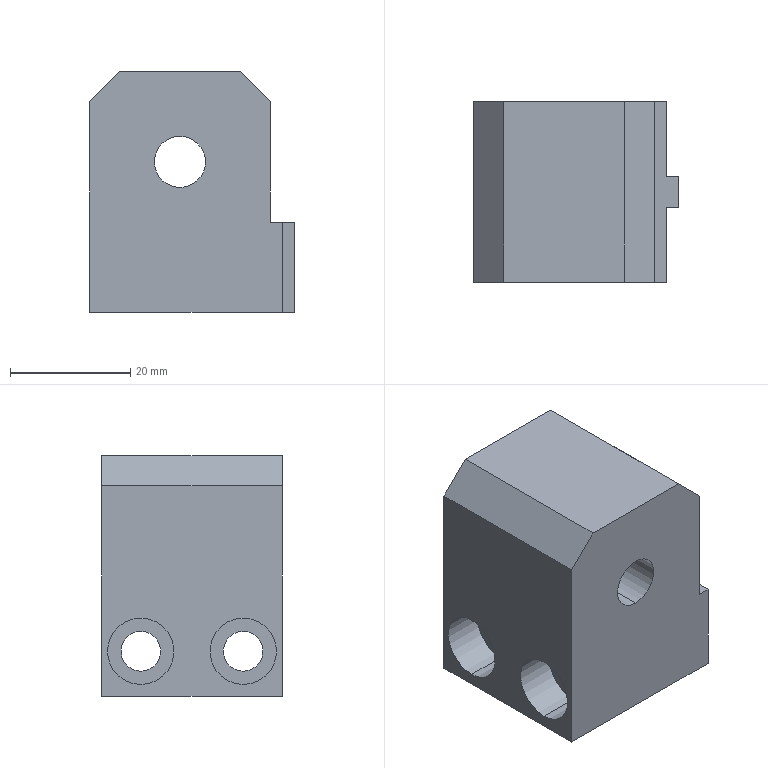Part | SolidWorks | features BaseBody 1 | 1 solid | 26 faces | box 34 x 30 x 40 mm | volume 31581 mm3 | plane 16 | cylinder 10 | commonest cylinder face diameters 6.6 x4 11 x4 8.5 x2
STEP:
#1=CARTESIAN_POINT('',(-34.,30.,35.));
#2=VERTEX_POINT('',#1);
#3=CARTESIAN_POINT('',(-29.,30.,40.));
#4=VERTEX_POINT('',#3);
#5=CARTESIAN_POINT('',(-29.,30.,40.));
#6=DIRECTION('',(0.7071,0.,0.7071));
#7=VECTOR('',#6,1000.);
#8=LINE('',#5,#7);
#9=EDGE_CURVE('',#2,#4,#8,.T.);
#10=ORIENTED_EDGE('',*,*,#9,.F.);
#11=CARTESIAN_POINT('',(-34.,0.,35.));
#12=VERTEX_POINT('',#11);
#13=CARTESIAN_POINT('',(-34.,30.,35.));
#14=DIRECTION('',(0.,1.,0.));
#15=VECTOR('',#14,1000.);
#16=LINE('',#13,#15);
#17=EDGE_CURVE('',#12,#2,#16,.T.);
#18=ORIENTED_EDGE('',*,*,#17,.F.);
#19=CARTESIAN_POINT('',(-29.,0.,40.));
#20=VERTEX_POINT('',#19);
#21=CARTESIAN_POINT('',(-34.5,0.,34.5));
#22=DIRECTION('',(-0.7071,0.,-0.7071));
#23=VECTOR('',#22,1000.);
#24=LINE('',#21,#23);
#25=EDGE_CURVE('',#20,#12,#24,.T.);
#26=ORIENTED_EDGE('',*,*,#25,.F.);
#27=CARTESIAN_POINT('',(-29.,30.,40.));
#28=DIRECTION('',(0.,-1.,0.));
#29=VECTOR('',#28,1000.);
#30=LINE('',#27,#29);
#31=EDGE_CURVE('',#4,#20,#30,.T.);
#32=ORIENTED_EDGE('',*,*,#31,.F.);
#33=EDGE_LOOP('',(#10,#18,#26,#32));
#34=FACE_OUTER_BOUND('',#33,.T.);
#35=CARTESIAN_POINT('',(-29.,30.,40.));
#36=DIRECTION('',(0.7071,0.,-0.7071));
#37=DIRECTION('',(0.,-1.,0.));
#38=AXIS2_PLACEMENT_3D('',#35,#36,#37);
#39=PLANE('',#38);
#40=ADVANCED_FACE('',(#34),#39,.F.);
#41=CARTESIAN_POINT('',(-9.,30.,40.));
#42=VERTEX_POINT('',#41);
#43=CARTESIAN_POINT('',(-4.,30.,35.));
#44=VERTEX_POINT('',#43);
#45=CARTESIAN_POINT('',(-4.,30.,35.));
#46=DIRECTION('',(0.7071,0.,-0.7071));
#47=VECTOR('',#46,1000.);
#48=LINE('',#45,#47);
#49=EDGE_CURVE('',#42,#44,#48,.T.);
#50=ORIENTED_EDGE('',*,*,#49,.F.);
#51=CARTESIAN_POINT('',(-9.,0.,40.));
#52=VERTEX_POINT('',#51);
#53=CARTESIAN_POINT('',(-9.,30.,40.));
#54=DIRECTION('',(0.,1.,0.));
#55=VECTOR('',#54,1000.);
#56=LINE('',#53,#55);
#57=EDGE_CURVE('',#52,#42,#56,.T.);
#58=ORIENTED_EDGE('',*,*,#57,.F.);
#59=CARTESIAN_POINT('',(-4.,0.,35.));
#60=VERTEX_POINT('',#59);
#61=CARTESIAN_POINT('',(15.5,0.,15.5));
#62=DIRECTION('',(-0.7071,0.,0.7071));
#63=VECTOR('',#62,1000.);
#64=LINE('',#61,#63);
#65=EDGE_CURVE('',#60,#52,#64,.T.);
#66=ORIENTED_EDGE('',*,*,#65,.F.);
#67=CARTESIAN_POINT('',(-4.,30.,35.));
#68=DIRECTION('',(0.,-1.,0.));
#69=VECTOR('',#68,1000.);
#70=LINE('',#67,#69);
#71=EDGE_CURVE('',#44,#60,#70,.T.);
#72=ORIENTED_EDGE('',*,*,#71,.F.);
#73=EDGE_LOOP('',(#50,#58,#66,#72));
#74=FACE_OUTER_BOUND('',#73,.T.);
#75=CARTESIAN_POINT('',(-4.,30.,35.));
#76=DIRECTION('',(-0.7071,0.,-0.7071));
#77=DIRECTION('',(-0.7071,0.,0.7071));
#78=AXIS2_PLACEMENT_3D('',#75,#76,#77);
#79=PLANE('',#78);
#80=ADVANCED_FACE('',(#74),#79,.F.);
#81=CARTESIAN_POINT('',(-27.2,23.5,2.));
#82=VERTEX_POINT('',#81);
#83=CARTESIAN_POINT('',(-34.,23.5,2.));
#84=VERTEX_POINT('',#83);
#85=CARTESIAN_POINT('',(-34.,23.5,2.));
#86=DIRECTION('',(-1.,0.,0.));
#87=VECTOR('',#86,1000.);
#88=LINE('',#85,#87);
#89=EDGE_CURVE('',#82,#84,#88,.T.);
#90=ORIENTED_EDGE('',*,*,#89,.F.);
#91=CARTESIAN_POINT('',(-27.2,23.5,13.));
#92=VERTEX_POINT('',#91);
#93=CARTESIAN_POINT('',(-27.2,23.5,7.5));
#94=DIRECTION('',(-1.,0.,0.));
#95=DIRECTION('',(0.,0.,1.));
#96=AXIS2_PLACEMENT_3D('',#93,#94,#95);
#97=CIRCLE('',#96,5.5);
#98=EDGE_CURVE('',#92,#82,#97,.T.);
#99=ORIENTED_EDGE('',*,*,#98,.F.);
#100=CARTESIAN_POINT('',(-34.,23.5,13.));
#101=VERTEX_POINT('',#100);
#102=CARTESIAN_POINT('',(-34.,23.5,13.));
#103=DIRECTION('',(-1.,0.,0.));
#104=VECTOR('',#103,1000.);
#105=LINE('',#102,#104);
#106=EDGE_CURVE('',#92,#101,#105,.T.);
#107=ORIENTED_EDGE('',*,*,#106,.T.);
#108=CARTESIAN_POINT('',(-34.,23.5,7.5));
#109=DIRECTION('',(-1.,0.,0.));
#110=DIRECTION('',(0.,0.,1.));
#111=AXIS2_PLACEMENT_3D('',#108,#109,#110);
#112=CIRCLE('',#111,5.5);
#113=EDGE_CURVE('',#101,#84,#112,.T.);
#114=ORIENTED_EDGE('',*,*,#113,.T.);
#115=EDGE_LOOP('',(#90,#99,#107,#114));
#116=FACE_OUTER_BOUND('',#115,.T.);
#117=CARTESIAN_POINT('',(-34.,23.5,7.5));
#118=DIRECTION('',(-1.,0.,0.));
#119=DIRECTION('',(0.,0.,1.));
#120=AXIS2_PLACEMENT_3D('',#117,#118,#119);
#121=CYLINDRICAL_SURFACE('',#120,5.5);
#122=ADVANCED_FACE('',(#116),#121,.F.);
#123=CARTESIAN_POINT('',(-27.2,23.5,10.8));
#124=VERTEX_POINT('',#123);
#125=CARTESIAN_POINT('',(-27.2,23.5,4.2));
#126=VERTEX_POINT('',#125);
#127=CARTESIAN_POINT('',(-27.2,23.5,7.5));
#128=DIRECTION('',(-1.,0.,0.));
#129=DIRECTION('',(0.,0.,1.));
#130=AXIS2_PLACEMENT_3D('',#127,#128,#129);
#131=CIRCLE('',#130,3.3);
#132=EDGE_CURVE('',#124,#126,#131,.T.);
#133=ORIENTED_EDGE('',*,*,#132,.F.);
#134=CARTESIAN_POINT('',(-27.2,23.5,7.5));
#135=DIRECTION('',(-1.,0.,0.));
#136=DIRECTION('',(0.,0.,1.));
#137=AXIS2_PLACEMENT_3D('',#134,#135,#136);
#138=CIRCLE('',#137,3.3);
#139=EDGE_CURVE('',#126,#124,#138,.T.);
#140=ORIENTED_EDGE('',*,*,#139,.F.);
#141=EDGE_LOOP('',(#133,#140));
#142=FACE_BOUND('',#141,.T.);
#143=ORIENTED_EDGE('',*,*,#98,.T.);
#144=CARTESIAN_POINT('',(-27.2,23.5,7.5));
#145=DIRECTION('',(-1.,0.,0.));
#146=DIRECTION('',(0.,0.,1.));
#147=AXIS2_PLACEMENT_3D('',#144,#145,#146);
#148=CIRCLE('',#147,5.5);
#149=EDGE_CURVE('',#82,#92,#148,.T.);
#150=ORIENTED_EDGE('',*,*,#149,.T.);
#151=EDGE_LOOP('',(#143,#150));
#152=FACE_OUTER_BOUND('',#151,.T.);
#153=CARTESIAN_POINT('',(-27.2,26.8,7.5));
#154=DIRECTION('',(1.,0.,0.));
#155=DIRECTION('',(0.,0.,-1.));
#156=AXIS2_PLACEMENT_3D('',#153,#154,#155);
#157=PLANE('',#156);
#158=ADVANCED_FACE('',(#142,#152),#157,.F.);
#159=CARTESIAN_POINT('',(-2.,23.5,4.2));
#160=VERTEX_POINT('',#159);
#161=CARTESIAN_POINT('',(-34.,23.5,4.2));
#162=DIRECTION('',(-1.,0.,0.));
#163=VECTOR('',#162,1000.);
#164=LINE('',#161,#163);
#165=EDGE_CURVE('',#160,#126,#164,.T.);
#166=ORIENTED_EDGE('',*,*,#165,.F.);
#167=CARTESIAN_POINT('',(-2.,23.5,10.8));
#168=VERTEX_POINT('',#167);
#169=CARTESIAN_POINT('',(-2.,23.5,7.5));
#170=DIRECTION('',(1.,0.,0.));
#171=DIRECTION('',(0.,0.,-1.));
#172=AXIS2_PLACEMENT_3D('',#169,#170,#171);
#173=CIRCLE('',#172,3.3);
#174=EDGE_CURVE('',#160,#168,#173,.T.);
#175=ORIENTED_EDGE('',*,*,#174,.T.);
#176=CARTESIAN_POINT('',(-34.,23.5,10.8));
#177=DIRECTION('',(-1.,0.,0.));
#178=VECTOR('',#177,1000.);
#179=LINE('',#176,#178);
#180=EDGE_CURVE('',#168,#124,#179,.T.);
#181=ORIENTED_EDGE('',*,*,#180,.T.);
#182=ORIENTED_EDGE('',*,*,#132,.T.);
#183=EDGE_LOOP('',(#166,#175,#181,#182));
#184=FACE_OUTER_BOUND('',#183,.T.);
#185=CARTESIAN_POINT('',(-34.,23.5,7.5));
#186=DIRECTION('',(-1.,0.,0.));
#187=DIRECTION('',(0.,0.,1.));
#188=AXIS2_PLACEMENT_3D('',#185,#186,#187);
#189=CYLINDRICAL_SURFACE('',#188,3.3);
#190=ADVANCED_FACE('',(#184),#189,.F.);
#191=CARTESIAN_POINT('',(-27.2,6.5,2.));
#192=VERTEX_POINT('',#191);
#193=CARTESIAN_POINT('',(-34.,6.5,2.));
#194=VERTEX_POINT('',#193);
#195=CARTESIAN_POINT('',(-34.,6.5,2.));
#196=DIRECTION('',(-1.,0.,0.));
#197=VECTOR('',#196,1000.);
#198=LINE('',#195,#197);
#199=EDGE_CURVE('',#192,#194,#198,.T.);
#200=ORIENTED_EDGE('',*,*,#199,.F.);
#201=CARTESIAN_POINT('',(-27.2,6.5,13.));
#202=VERTEX_POINT('',#201);
#203=CARTESIAN_POINT('',(-27.2,6.5,7.5));
#204=DIRECTION('',(-1.,0.,0.));
#205=DIRECTION('',(0.,0.,1.));
#206=AXIS2_PLACEMENT_3D('',#203,#204,#205);
#207=CIRCLE('',#206,5.5);
#208=EDGE_CURVE('',#202,#192,#207,.T.);
#209=ORIENTED_EDGE('',*,*,#208,.F.);
#210=CARTESIAN_POINT('',(-34.,6.5,13.));
#211=VERTEX_POINT('',#210);
#212=CARTESIAN_POINT('',(-34.,6.5,13.));
#213=DIRECTION('',(-1.,0.,0.));
#214=VECTOR('',#213,1000.);
#215=LINE('',#212,#214);
#216=EDGE_CURVE('',#202,#211,#215,.T.);
#217=ORIENTED_EDGE('',*,*,#216,.T.);
#218=CARTESIAN_POINT('',(-34.,6.5,7.5));
#219=DIRECTION('',(-1.,0.,0.));
#220=DIRECTION('',(0.,0.,1.));
#221=AXIS2_PLACEMENT_3D('',#218,#219,#220);
#222=CIRCLE('',#221,5.5);
#223=EDGE_CURVE('',#211,#194,#222,.T.);
#224=ORIENTED_EDGE('',*,*,#223,.T.);
#225=EDGE_LOOP('',(#200,#209,#217,#224));
#226=FACE_OUTER_BOUND('',#225,.T.);
#227=CARTESIAN_POINT('',(-34.,6.5,7.5));
#228=DIRECTION('',(-1.,0.,0.));
#229=DIRECTION('',(0.,0.,1.));
#230=AXIS2_PLACEMENT_3D('',#227,#228,#229);
#231=CYLINDRICAL_SURFACE('',#230,5.5);
#232=ADVANCED_FACE('',(#226),#231,.F.);
#233=CARTESIAN_POINT('',(-27.2,6.5,10.8));
#234=VERTEX_POINT('',#233);
#235=CARTESIAN_POINT('',(-27.2,6.5,4.2));
#236=VERTEX_POINT('',#235);
#237=CARTESIAN_POINT('',(-27.2,6.5,7.5));
#238=DIRECTION('',(-1.,0.,0.));
#239=DIRECTION('',(0.,0.,1.));
#240=AXIS2_PLACEMENT_3D('',#237,#238,#239);
#241=CIRCLE('',#240,3.3);
#242=EDGE_CURVE('',#234,#236,#241,.T.);
#243=ORIENTED_EDGE('',*,*,#242,.F.);
#244=CARTESIAN_POINT('',(-27.2,6.5,7.5));
#245=DIRECTION('',(-1.,0.,0.));
#246=DIRECTION('',(0.,0.,1.));
#247=AXIS2_PLACEMENT_3D('',#244,#245,#246);
#248=CIRCLE('',#247,3.3);
#249=EDGE_CURVE('',#236,#234,#248,.T.);
#250=ORIENTED_EDGE('',*,*,#249,.F.);
#251=EDGE_LOOP('',(#243,#250));
#252=FACE_BOUND('',#251,.T.);
#253=ORIENTED_EDGE('',*,*,#208,.T.);
#254=CARTESIAN_POINT('',(-27.2,6.5,7.5));
#255=DIRECTION('',(-1.,0.,0.));
#256=DIRECTION('',(0.,0.,1.));
#257=AXIS2_PLACEMENT_3D('',#254,#255,#256);
#258=CIRCLE('',#257,5.5);
#259=EDGE_CURVE('',#192,#202,#258,.T.);
#260=ORIENTED_EDGE('',*,*,#259,.T.);
#261=EDGE_LOOP('',(#253,#260));
#262=FACE_OUTER_BOUND('',#261,.T.);
#263=CARTESIAN_POINT('',(-27.2,9.8,7.5));
#264=DIRECTION('',(1.,0.,0.));
#265=DIRECTION('',(0.,0.,-1.));
#266=AXIS2_PLACEMENT_3D('',#263,#264,#265);
#267=PLANE('',#266);
#268=ADVANCED_FACE('',(#252,#262),#267,.F.);
#269=CARTESIAN_POINT('',(-2.,6.5,4.2));
#270=VERTEX_POINT('',#269);
#271=CARTESIAN_POINT('',(-34.,6.5,4.2));
#272=DIRECTION('',(-1.,0.,0.));
#273=VECTOR('',#272,1000.);
#274=LINE('',#271,#273);
#275=EDGE_CURVE('',#270,#236,#274,.T.);
#276=ORIENTED_EDGE('',*,*,#275,.F.);
#277=CARTESIAN_POINT('',(-2.,6.5,10.8));
#278=VERTEX_POINT('',#277);
#279=CARTESIAN_POINT('',(-2.,6.5,7.5));
#280=DIRECTION('',(1.,0.,0.));
#281=DIRECTION('',(0.,0.,-1.));
#282=AXIS2_PLACEMENT_3D('',#279,#280,#281);
#283=CIRCLE('',#282,3.3);
#284=EDGE_CURVE('',#270,#278,#283,.T.);
#285=ORIENTED_EDGE('',*,*,#284,.T.);
#286=CARTESIAN_POINT('',(-34.,6.5,10.8));
#287=DIRECTION('',(-1.,0.,0.));
#288=VECTOR('',#287,1000.);
#289=LINE('',#286,#288);
#290=EDGE_CURVE('',#278,#234,#289,.T.);
#291=ORIENTED_EDGE('',*,*,#290,.T.);
#292=ORIENTED_EDGE('',*,*,#242,.T.);
#293=EDGE_LOOP('',(#276,#285,#291,#292));
#294=FACE_OUTER_BOUND('',#293,.T.);
#295=CARTESIAN_POINT('',(-34.,6.5,7.5));
#296=DIRECTION('',(-1.,0.,0.));
#297=DIRECTION('',(0.,0.,1.));
#298=AXIS2_PLACEMENT_3D('',#295,#296,#297);
#299=CYLINDRICAL_SURFACE('',#298,3.3);
#300=ADVANCED_FACE('',(#294),#299,.F.);
#301=CARTESIAN_POINT('',(-2.,23.5,7.5));
#302=DIRECTION('',(1.,0.,0.));
#303=DIRECTION('',(0.,0.,-1.));
#304=AXIS2_PLACEMENT_3D('',#301,#302,#303);
#305=CIRCLE('',#304,3.3);
#306=EDGE_CURVE('',#168,#160,#305,.T.);
#307=ORIENTED_EDGE('',*,*,#306,.F.);
#308=ORIENTED_EDGE('',*,*,#174,.F.);
#309=EDGE_LOOP('',(#307,#308));
#310=FACE_BOUND('',#309,.T.);
#311=CARTESIAN_POINT('',(-2.,30.,15.));
#312=VERTEX_POINT('',#311);
#313=CARTESIAN_POINT('',(-2.,17.5,15.));
#314=VERTEX_POINT('',#313);
#315=CARTESIAN_POINT('',(-2.,30.,15.));
#316=DIRECTION('',(0.,-1.,0.));
#317=VECTOR('',#316,1000.);
#318=LINE('',#315,#317);
#319=EDGE_CURVE('',#312,#314,#318,.T.);
#320=ORIENTED_EDGE('',*,*,#319,.T.);
#321=CARTESIAN_POINT('',(-2.,17.5,0.));
#322=VERTEX_POINT('',#321);
#323=CARTESIAN_POINT('',(-2.,17.5,15.));
#324=DIRECTION('',(0.,0.,-1.));
#325=VECTOR('',#324,1000.);
#326=LINE('',#323,#325);
#327=EDGE_CURVE('',#314,#322,#326,.T.);
#328=ORIENTED_EDGE('',*,*,#327,.T.);
#329=CARTESIAN_POINT('',(-2.,30.,0.));
#330=VERTEX_POINT('',#329);
#331=CARTESIAN_POINT('',(-2.,30.,0.));
#332=DIRECTION('',(0.,1.,0.));
#333=VECTOR('',#332,1000.);
#334=LINE('',#331,#333);
#335=EDGE_CURVE('',#322,#330,#334,.T.);
#336=ORIENTED_EDGE('',*,*,#335,.T.);
#337=CARTESIAN_POINT('',(-2.,30.,15.));
#338=DIRECTION('',(0.,0.,1.));
#339=VECTOR('',#338,1000.);
#340=LINE('',#337,#339);
#341=EDGE_CURVE('',#330,#312,#340,.T.);
#342=ORIENTED_EDGE('',*,*,#341,.T.);
#343=EDGE_LOOP('',(#320,#328,#336,#342));
#344=FACE_OUTER_BOUND('',#343,.T.);
#345=CARTESIAN_POINT('',(-2.,0.,0.));
#346=DIRECTION('',(1.,0.,0.));
#347=DIRECTION('',(0.,0.,-1.));
#348=AXIS2_PLACEMENT_3D('',#345,#346,#347);
#349=PLANE('',#348);
#350=ADVANCED_FACE('',(#310,#344),#349,.T.);
#351=CARTESIAN_POINT('',(0.,17.5,15.));
#352=VERTEX_POINT('',#351);
#353=CARTESIAN_POINT('',(0.,17.5,0.));
#354=VERTEX_POINT('',#353);
#355=CARTESIAN_POINT('',(0.,17.5,15.));
#356=DIRECTION('',(0.,0.,-1.));
#357=VECTOR('',#356,1000.);
#358=LINE('',#355,#357);
#359=EDGE_CURVE('',#352,#354,#358,.T.);
#360=ORIENTED_EDGE('',*,*,#359,.T.);
#361=CARTESIAN_POINT('',(-2.,17.5,0.));
#362=DIRECTION('',(1.,0.,0.));
#363=VECTOR('',#362,1000.);
#364=LINE('',#361,#363);
#365=EDGE_CURVE('',#322,#354,#364,.T.);
#366=ORIENTED_EDGE('',*,*,#365,.F.);
#367=ORIENTED_EDGE('',*,*,#327,.F.);
#368=CARTESIAN_POINT('',(-2.,17.5,15.));
#369=DIRECTION('',(1.,0.,0.));
#370=VECTOR('',#369,1000.);
#371=LINE('',#368,#370);
#372=EDGE_CURVE('',#314,#352,#371,.T.);
#373=ORIENTED_EDGE('',*,*,#372,.T.);
#374=EDGE_LOOP('',(#360,#366,#367,#373));
#375=FACE_OUTER_BOUND('',#374,.T.);
#376=CARTESIAN_POINT('',(-2.,17.5,15.));
#377=DIRECTION('',(0.,-1.,0.));
#378=DIRECTION('',(0.,0.,-1.));
#379=AXIS2_PLACEMENT_3D('',#376,#377,#378);
#380=PLANE('',#379);
#381=ADVANCED_FACE('',(#375),#380,.F.);
#382=CARTESIAN_POINT('',(-2.,6.5,7.5));
#383=DIRECTION('',(1.,0.,0.));
#384=DIRECTION('',(0.,0.,-1.));
#385=AXIS2_PLACEMENT_3D('',#382,#383,#384);
#386=CIRCLE('',#385,3.3);
#387=EDGE_CURVE('',#278,#270,#386,.T.);
#388=ORIENTED_EDGE('',*,*,#387,.F.);
#389=ORIENTED_EDGE('',*,*,#284,.F.);
#390=EDGE_LOOP('',(#388,#389));
#391=FACE_BOUND('',#390,.T.);
#392=CARTESIAN_POINT('',(-2.,0.,15.));
#393=VERTEX_POINT('',#392);
#394=CARTESIAN_POINT('',(-2.,0.,0.));
#395=VERTEX_POINT('',#394);
#396=CARTESIAN_POINT('',(-2.,0.,15.));
#397=DIRECTION('',(0.,0.,-1.));
#398=VECTOR('',#397,1000.);
#399=LINE('',#396,#398);
#400=EDGE_CURVE('',#393,#395,#399,.T.);
#401=ORIENTED_EDGE('',*,*,#400,.T.);
#402=CARTESIAN_POINT('',(-2.,12.5,0.));
#403=VERTEX_POINT('',#402);
#404=CARTESIAN_POINT('',(-2.,0.,0.));
#405=DIRECTION('',(0.,1.,0.));
#406=VECTOR('',#405,1000.);
#407=LINE('',#404,#406);
#408=EDGE_CURVE('',#395,#403,#407,.T.);
#409=ORIENTED_EDGE('',*,*,#408,.T.);
#410=CARTESIAN_POINT('',(-2.,12.5,15.));
#411=VERTEX_POINT('',#410);
#412=CARTESIAN_POINT('',(-2.,12.5,15.));
#413=DIRECTION('',(0.,0.,1.));
#414=VECTOR('',#413,1000.);
#415=LINE('',#412,#414);
#416=EDGE_CURVE('',#403,#411,#415,.T.);
#417=ORIENTED_EDGE('',*,*,#416,.T.);
#418=CARTESIAN_POINT('',(-2.,0.,15.));
#419=DIRECTION('',(0.,-1.,0.));
#420=VECTOR('',#419,1000.);
#421=LINE('',#418,#420);
#422=EDGE_CURVE('',#411,#393,#421,.T.);
#423=ORIENTED_EDGE('',*,*,#422,.T.);
#424=EDGE_LOOP('',(#401,#409,#417,#423));
#425=FACE_OUTER_BOUND('',#424,.T.);
#426=CARTESIAN_POINT('',(-2.,0.,0.));
#427=DIRECTION('',(1.,0.,0.));
#428=DIRECTION('',(0.,0.,-1.));
#429=AXIS2_PLACEMENT_3D('',#426,#427,#428);
#430=PLANE('',#429);
#431=ADVANCED_FACE('',(#391,#425),#430,.T.);
#432=CARTESIAN_POINT('',(0.,12.5,0.));
#433=VERTEX_POINT('',#432);
#434=CARTESIAN_POINT('',(0.,12.5,15.));
#435=VERTEX_POINT('',#434);
#436=CARTESIAN_POINT('',(0.,12.5,15.));
#437=DIRECTION('',(0.,0.,1.));
#438=VECTOR('',#437,1000.);
#439=LINE('',#436,#438);
#440=EDGE_CURVE('',#433,#435,#439,.T.);
#441=ORIENTED_EDGE('',*,*,#440,.T.);
#442=CARTESIAN_POINT('',(-2.,12.5,15.));
#443=DIRECTION('',(1.,0.,0.));
#444=VECTOR('',#443,1000.);
#445=LINE('',#442,#444);
#446=EDGE_CURVE('',#411,#435,#445,.T.);
#447=ORIENTED_EDGE('',*,*,#446,.F.);
#448=ORIENTED_EDGE('',*,*,#416,.F.);
#449=CARTESIAN_POINT('',(-2.,12.5,0.));
#450=DIRECTION('',(1.,0.,0.));
#451=VECTOR('',#450,1000.);
#452=LINE('',#449,#451);
#453=EDGE_CURVE('',#403,#433,#452,.T.);
#454=ORIENTED_EDGE('',*,*,#453,.T.);
#455=EDGE_LOOP('',(#441,#447,#448,#454));
#456=FACE_OUTER_BOUND('',#455,.T.);
#457=CARTESIAN_POINT('',(-2.,12.5,15.));
#458=DIRECTION('',(0.,1.,0.));
#459=DIRECTION('',(0.,0.,-1.));
#460=AXIS2_PLACEMENT_3D('',#457,#458,#459);
#461=PLANE('',#460);
#462=ADVANCED_FACE('',(#456),#461,.F.);
#463=CARTESIAN_POINT('',(-19.,0.,20.75));
#464=VERTEX_POINT('',#463);
#465=CARTESIAN_POINT('',(-19.,30.,20.75));
#466=VERTEX_POINT('',#465);
#467=CARTESIAN_POINT('',(-19.,30.,20.75));
#468=DIRECTION('',(0.,1.,0.));
#469=VECTOR('',#468,1000.);
#470=LINE('',#467,#469);
#471=EDGE_CURVE('',#464,#466,#470,.T.);
#472=ORIENTED_EDGE('',*,*,#471,.F.);
#473=CARTESIAN_POINT('',(-19.,0.,29.25));
#474=VERTEX_POINT('',#473);
#475=CARTESIAN_POINT('',(-19.,0.,25.));
#476=DIRECTION('',(0.,1.,0.));
#477=DIRECTION('',(0.,0.,1.));
#478=AXIS2_PLACEMENT_3D('',#475,#476,#477);
#479=CIRCLE('',#478,4.25);
#480=EDGE_CURVE('',#474,#464,#479,.T.);
#481=ORIENTED_EDGE('',*,*,#480,.F.);
#482=CARTESIAN_POINT('',(-19.,30.,29.25));
#483=VERTEX_POINT('',#482);
#484=CARTESIAN_POINT('',(-19.,30.,29.25));
#485=DIRECTION('',(0.,1.,0.));
#486=VECTOR('',#485,1000.);
#487=LINE('',#484,#486);
#488=EDGE_CURVE('',#474,#483,#487,.T.);
#489=ORIENTED_EDGE('',*,*,#488,.T.);
#490=CARTESIAN_POINT('',(-19.,30.,25.));
#491=DIRECTION('',(0.,1.,0.));
#492=DIRECTION('',(0.,0.,1.));
#493=AXIS2_PLACEMENT_3D('',#490,#491,#492);
#494=CIRCLE('',#493,4.25);
#495=EDGE_CURVE('',#483,#466,#494,.T.);
#496=ORIENTED_EDGE('',*,*,#495,.T.);
#497=EDGE_LOOP('',(#472,#481,#489,#496));
#498=FACE_OUTER_BOUND('',#497,.T.);
#499=CARTESIAN_POINT('',(-19.,30.,25.));
#500=DIRECTION('',(0.,1.,0.));
#501=DIRECTION('',(0.,0.,1.));
#502=AXIS2_PLACEMENT_3D('',#499,#500,#501);
#503=CYLINDRICAL_SURFACE('',#502,4.25);
#504=ADVANCED_FACE('',(#498),#503,.F.);
#505=CARTESIAN_POINT('',(0.,30.,15.));
#506=DIRECTION('',(0.,-1.,0.));
#507=VECTOR('',#506,1000.);
#508=LINE('',#505,#507);
#509=EDGE_CURVE('',#352,#435,#508,.T.);
#510=ORIENTED_EDGE('',*,*,#509,.F.);
#511=ORIENTED_EDGE('',*,*,#372,.F.);
#512=ORIENTED_EDGE('',*,*,#319,.F.);
#513=CARTESIAN_POINT('',(-4.,30.,15.));
#514=VERTEX_POINT('',#513);
#515=CARTESIAN_POINT('',(0.,30.,15.));
#516=DIRECTION('',(1.,0.,0.));
#517=VECTOR('',#516,1000.);
#518=LINE('',#515,#517);
#519=EDGE_CURVE('',#514,#312,#518,.T.);
#520=ORIENTED_EDGE('',*,*,#519,.F.);
#521=CARTESIAN_POINT('',(-4.,0.,15.));
#522=VERTEX_POINT('',#521);
#523=CARTESIAN_POINT('',(-4.,30.,15.));
#524=DIRECTION('',(0.,-1.,0.));
#525=VECTOR('',#524,1000.);
#526=LINE('',#523,#525);
#527=EDGE_CURVE('',#514,#522,#526,.T.);
#528=ORIENTED_EDGE('',*,*,#527,.T.);
#529=CARTESIAN_POINT('',(0.,0.,15.));
#530=DIRECTION('',(1.,0.,0.));
#531=VECTOR('',#530,1000.);
#532=LINE('',#529,#531);
#533=EDGE_CURVE('',#522,#393,#532,.T.);
#534=ORIENTED_EDGE('',*,*,#533,.T.);
#535=ORIENTED_EDGE('',*,*,#422,.F.);
#536=ORIENTED_EDGE('',*,*,#446,.T.);
#537=EDGE_LOOP('',(#510,#511,#512,#520,#528,#534,#535,#536));
#538=FACE_OUTER_BOUND('',#537,.T.);
#539=CARTESIAN_POINT('',(0.,30.,15.));
#540=DIRECTION('',(0.,0.,-1.));
#541=DIRECTION('',(0.,-1.,0.));
#542=AXIS2_PLACEMENT_3D('',#539,#540,#541);
#543=PLANE('',#542);
#544=ADVANCED_FACE('',(#538),#543,.F.);
#545=CARTESIAN_POINT('',(-4.,30.,15.));
#546=DIRECTION('',(0.,0.,-1.));
#547=VECTOR('',#546,1000.);
#548=LINE('',#545,#547);
#549=EDGE_CURVE('',#44,#514,#548,.T.);
#550=ORIENTED_EDGE('',*,*,#549,.F.);
#551=ORIENTED_EDGE('',*,*,#71,.T.);
#552=CARTESIAN_POINT('',(-4.,0.,15.));
#553=DIRECTION('',(0.,0.,-1.));
#554=VECTOR('',#553,1000.);
#555=LINE('',#552,#554);
#556=EDGE_CURVE('',#60,#522,#555,.T.);
#557=ORIENTED_EDGE('',*,*,#556,.T.);
#558=ORIENTED_EDGE('',*,*,#527,.F.);
#559=EDGE_LOOP('',(#550,#551,#557,#558));
#560=FACE_OUTER_BOUND('',#559,.T.);
#561=CARTESIAN_POINT('',(-4.,30.,15.));
#562=DIRECTION('',(-1.,0.,0.));
#563=DIRECTION('',(0.,1.,0.));
#564=AXIS2_PLACEMENT_3D('',#561,#562,#563);
#565=PLANE('',#564);
#566=ADVANCED_FACE('',(#560),#565,.F.);
#567=CARTESIAN_POINT('',(-34.,0.,40.));
#568=DIRECTION('',(1.,0.,0.));
#569=VECTOR('',#568,1000.);
#570=LINE('',#567,#569);
#571=EDGE_CURVE('',#20,#52,#570,.T.);
#572=ORIENTED_EDGE('',*,*,#571,.T.);
#573=ORIENTED_EDGE('',*,*,#57,.T.);
#574=CARTESIAN_POINT('',(-34.,30.,40.));
#575=DIRECTION('',(1.,0.,0.));
#576=VECTOR('',#575,1000.);
#577=LINE('',#574,#576);
#578=EDGE_CURVE('',#4,#42,#577,.T.);
#579=ORIENTED_EDGE('',*,*,#578,.F.);
#580=ORIENTED_EDGE('',*,*,#31,.T.);
#581=EDGE_LOOP('',(#572,#573,#579,#580));
#582=FACE_OUTER_BOUND('',#581,.T.);
#583=CARTESIAN_POINT('',(-34.,30.,40.));
#584=DIRECTION('',(0.,0.,-1.));
#585=DIRECTION('',(0.,-1.,0.));
#586=AXIS2_PLACEMENT_3D('',#583,#584,#585);
#587=PLANE('',#586);
#588=ADVANCED_FACE('',(#582),#587,.F.);
#589=ORIENTED_EDGE('',*,*,#223,.F.);
#590=CARTESIAN_POINT('',(-34.,6.5,7.5));
#591=DIRECTION('',(-1.,0.,0.));
#592=DIRECTION('',(0.,0.,1.));
#593=AXIS2_PLACEMENT_3D('',#590,#591,#592);
#594=CIRCLE('',#593,5.5);
#595=EDGE_CURVE('',#194,#211,#594,.T.);
#596=ORIENTED_EDGE('',*,*,#595,.F.);
#597=EDGE_LOOP('',(#589,#596));
#598=FACE_BOUND('',#597,.T.);
#599=ORIENTED_EDGE('',*,*,#113,.F.);
#600=CARTESIAN_POINT('',(-34.,23.5,7.5));
#601=DIRECTION('',(-1.,0.,0.));
#602=DIRECTION('',(0.,0.,1.));
#603=AXIS2_PLACEMENT_3D('',#600,#601,#602);
#604=CIRCLE('',#603,5.5);
#605=EDGE_CURVE('',#84,#101,#604,.T.);
#606=ORIENTED_EDGE('',*,*,#605,.F.);
#607=EDGE_LOOP('',(#599,#606));
#608=FACE_BOUND('',#607,.T.);
#609=CARTESIAN_POINT('',(-34.,0.,0.));
#610=VERTEX_POINT('',#609);
#611=CARTESIAN_POINT('',(-34.,0.,0.));
#612=DIRECTION('',(0.,0.,1.));
#613=VECTOR('',#612,1000.);
#614=LINE('',#611,#613);
#615=EDGE_CURVE('',#610,#12,#614,.T.);
#616=ORIENTED_EDGE('',*,*,#615,.T.);
#617=ORIENTED_EDGE('',*,*,#17,.T.);
#618=CARTESIAN_POINT('',(-34.,30.,0.));
#619=VERTEX_POINT('',#618);
#620=CARTESIAN_POINT('',(-34.,30.,0.));
#621=DIRECTION('',(0.,0.,1.));
#622=VECTOR('',#621,1000.);
#623=LINE('',#620,#622);
#624=EDGE_CURVE('',#619,#2,#623,.T.);
#625=ORIENTED_EDGE('',*,*,#624,.F.);
#626=CARTESIAN_POINT('',(-34.,30.,0.));
#627=DIRECTION('',(0.,-1.,0.));
#628=VECTOR('',#627,1000.);
#629=LINE('',#626,#628);
#630=EDGE_CURVE('',#619,#610,#629,.T.);
#631=ORIENTED_EDGE('',*,*,#630,.T.);
#632=EDGE_LOOP('',(#616,#617,#625,#631));
#633=FACE_OUTER_BOUND('',#632,.T.);
#634=CARTESIAN_POINT('',(-34.,30.,0.));
#635=DIRECTION('',(1.,0.,0.));
#636=DIRECTION('',(0.,0.,-1.));
#637=AXIS2_PLACEMENT_3D('',#634,#635,#636);
#638=PLANE('',#637);
#639=ADVANCED_FACE('',(#598,#608,#633),#638,.F.);
#640=ORIENTED_EDGE('',*,*,#335,.F.);
#641=ORIENTED_EDGE('',*,*,#365,.T.);
#642=CARTESIAN_POINT('',(0.,30.,0.));
#643=DIRECTION('',(0.,-1.,0.));
#644=VECTOR('',#643,1000.);
#645=LINE('',#642,#644);
#646=EDGE_CURVE('',#354,#433,#645,.T.);
#647=ORIENTED_EDGE('',*,*,#646,.T.);
#648=ORIENTED_EDGE('',*,*,#453,.F.);
#649=ORIENTED_EDGE('',*,*,#408,.F.);
#650=CARTESIAN_POINT('',(-34.,0.,0.));
#651=DIRECTION('',(-1.,0.,0.));
#652=VECTOR('',#651,1000.);
#653=LINE('',#650,#652);
#654=EDGE_CURVE('',#395,#610,#653,.T.);
#655=ORIENTED_EDGE('',*,*,#654,.T.);
#656=ORIENTED_EDGE('',*,*,#630,.F.);
#657=CARTESIAN_POINT('',(-34.,30.,0.));
#658=DIRECTION('',(-1.,0.,0.));
#659=VECTOR('',#658,1000.);
#660=LINE('',#657,#659);
#661=EDGE_CURVE('',#330,#619,#660,.T.);
#662=ORIENTED_EDGE('',*,*,#661,.F.);
#663=EDGE_LOOP('',(#640,#641,#647,#648,#649,#655,#656,#662));
#664=FACE_OUTER_BOUND('',#663,.T.);
#665=CARTESIAN_POINT('',(-34.,30.,0.));
#666=DIRECTION('',(0.,0.,1.));
#667=DIRECTION('',(1.,0.,0.));
#668=AXIS2_PLACEMENT_3D('',#665,#666,#667);
#669=PLANE('',#668);
#670=ADVANCED_FACE('',(#664),#669,.F.);
#671=ORIENTED_EDGE('',*,*,#646,.F.);
#672=ORIENTED_EDGE('',*,*,#359,.F.);
#673=ORIENTED_EDGE('',*,*,#509,.T.);
#674=ORIENTED_EDGE('',*,*,#440,.F.);
#675=EDGE_LOOP('',(#671,#672,#673,#674));
#676=FACE_OUTER_BOUND('',#675,.T.);
#677=CARTESIAN_POINT('',(0.,30.,0.));
#678=DIRECTION('',(-1.,0.,0.));
#679=DIRECTION('',(0.,1.,0.));
#680=AXIS2_PLACEMENT_3D('',#677,#678,#679);
#681=PLANE('',#680);
#682=ADVANCED_FACE('',(#676),#681,.F.);
#683=ORIENTED_EDGE('',*,*,#480,.T.);
#684=CARTESIAN_POINT('',(-19.,0.,25.));
#685=DIRECTION('',(0.,1.,0.));
#686=DIRECTION('',(0.,0.,1.));
#687=AXIS2_PLACEMENT_3D('',#684,#685,#686);
#688=CIRCLE('',#687,4.25);
#689=EDGE_CURVE('',#464,#474,#688,.T.);
#690=ORIENTED_EDGE('',*,*,#689,.T.);
#691=EDGE_LOOP('',(#683,#690));
#692=FACE_BOUND('',#691,.T.);
#693=ORIENTED_EDGE('',*,*,#556,.F.);
#694=ORIENTED_EDGE('',*,*,#65,.T.);
#695=ORIENTED_EDGE('',*,*,#571,.F.);
#696=ORIENTED_EDGE('',*,*,#25,.T.);
#697=ORIENTED_EDGE('',*,*,#615,.F.);
#698=ORIENTED_EDGE('',*,*,#654,.F.);
#699=ORIENTED_EDGE('',*,*,#400,.F.);
#700=ORIENTED_EDGE('',*,*,#533,.F.);
#701=EDGE_LOOP('',(#693,#694,#695,#696,#697,#698,#699,#700));
#702=FACE_OUTER_BOUND('',#701,.T.);
#703=CARTESIAN_POINT('',(0.,0.,0.));
#704=DIRECTION('',(0.,-1.,0.));
#705=DIRECTION('',(0.,0.,-1.));
#706=AXIS2_PLACEMENT_3D('',#703,#704,#705);
#707=PLANE('',#706);
#708=ADVANCED_FACE('',(#692,#702),#707,.T.);
#709=ORIENTED_EDGE('',*,*,#495,.F.);
#710=CARTESIAN_POINT('',(-19.,30.,25.));
#711=DIRECTION('',(0.,1.,0.));
#712=DIRECTION('',(0.,0.,1.));
#713=AXIS2_PLACEMENT_3D('',#710,#711,#712);
#714=CIRCLE('',#713,4.25);
#715=EDGE_CURVE('',#466,#483,#714,.T.);
#716=ORIENTED_EDGE('',*,*,#715,.F.);
#717=EDGE_LOOP('',(#709,#716));
#718=FACE_BOUND('',#717,.T.);
#719=ORIENTED_EDGE('',*,*,#578,.T.);
#720=ORIENTED_EDGE('',*,*,#49,.T.);
#721=ORIENTED_EDGE('',*,*,#549,.T.);
#722=ORIENTED_EDGE('',*,*,#519,.T.);
#723=ORIENTED_EDGE('',*,*,#341,.F.);
#724=ORIENTED_EDGE('',*,*,#661,.T.);
#725=ORIENTED_EDGE('',*,*,#624,.T.);
#726=ORIENTED_EDGE('',*,*,#9,.T.);
#727=EDGE_LOOP('',(#719,#720,#721,#722,#723,#724,#725,#726));
#728=FACE_OUTER_BOUND('',#727,.T.);
#729=CARTESIAN_POINT('',(0.,30.,0.));
#730=DIRECTION('',(0.,-1.,0.));
#731=DIRECTION('',(0.,0.,-1.));
#732=AXIS2_PLACEMENT_3D('',#729,#730,#731);
#733=PLANE('',#732);
#734=ADVANCED_FACE('',(#718,#728),#733,.F.);
#735=ORIENTED_EDGE('',*,*,#689,.F.);
#736=ORIENTED_EDGE('',*,*,#471,.T.);
#737=ORIENTED_EDGE('',*,*,#715,.T.);
#738=ORIENTED_EDGE('',*,*,#488,.F.);
#739=EDGE_LOOP('',(#735,#736,#737,#738));
#740=FACE_OUTER_BOUND('',#739,.T.);
#741=CARTESIAN_POINT('',(-19.,30.,25.));
#742=DIRECTION('',(0.,1.,0.));
#743=DIRECTION('',(0.,0.,1.));
#744=AXIS2_PLACEMENT_3D('',#741,#742,#743);
#745=CYLINDRICAL_SURFACE('',#744,4.25);
#746=ADVANCED_FACE('',(#740),#745,.F.);
#747=ORIENTED_EDGE('',*,*,#387,.T.);
#748=ORIENTED_EDGE('',*,*,#275,.T.);
#749=ORIENTED_EDGE('',*,*,#249,.T.);
#750=ORIENTED_EDGE('',*,*,#290,.F.);
#751=EDGE_LOOP('',(#747,#748,#749,#750));
#752=FACE_OUTER_BOUND('',#751,.T.);
#753=CARTESIAN_POINT('',(-34.,6.5,7.5));
#754=DIRECTION('',(-1.,0.,0.));
#755=DIRECTION('',(0.,0.,1.));
#756=AXIS2_PLACEMENT_3D('',#753,#754,#755);
#757=CYLINDRICAL_SURFACE('',#756,3.3);
#758=ADVANCED_FACE('',(#752),#757,.F.);
#759=ORIENTED_EDGE('',*,*,#259,.F.);
#760=ORIENTED_EDGE('',*,*,#199,.T.);
#761=ORIENTED_EDGE('',*,*,#595,.T.);
#762=ORIENTED_EDGE('',*,*,#216,.F.);
#763=EDGE_LOOP('',(#759,#760,#761,#762));
#764=FACE_OUTER_BOUND('',#763,.T.);
#765=CARTESIAN_POINT('',(-34.,6.5,7.5));
#766=DIRECTION('',(-1.,0.,0.));
#767=DIRECTION('',(0.,0.,1.));
#768=AXIS2_PLACEMENT_3D('',#765,#766,#767);
#769=CYLINDRICAL_SURFACE('',#768,5.5);
#770=ADVANCED_FACE('',(#764),#769,.F.);
#771=ORIENTED_EDGE('',*,*,#306,.T.);
#772=ORIENTED_EDGE('',*,*,#165,.T.);
#773=ORIENTED_EDGE('',*,*,#139,.T.);
#774=ORIENTED_EDGE('',*,*,#180,.F.);
#775=EDGE_LOOP('',(#771,#772,#773,#774));
#776=FACE_OUTER_BOUND('',#775,.T.);
#777=CARTESIAN_POINT('',(-34.,23.5,7.5));
#778=DIRECTION('',(-1.,0.,0.));
#779=DIRECTION('',(0.,0.,1.));
#780=AXIS2_PLACEMENT_3D('',#777,#778,#779);
#781=CYLINDRICAL_SURFACE('',#780,3.3);
#782=ADVANCED_FACE('',(#776),#781,.F.);
#783=ORIENTED_EDGE('',*,*,#149,.F.);
#784=ORIENTED_EDGE('',*,*,#89,.T.);
#785=ORIENTED_EDGE('',*,*,#605,.T.);
#786=ORIENTED_EDGE('',*,*,#106,.F.);
#787=EDGE_LOOP('',(#783,#784,#785,#786));
#788=FACE_OUTER_BOUND('',#787,.T.);
#789=CARTESIAN_POINT('',(-34.,23.5,7.5));
#790=DIRECTION('',(-1.,0.,0.));
#791=DIRECTION('',(0.,0.,1.));
#792=AXIS2_PLACEMENT_3D('',#789,#790,#791);
#793=CYLINDRICAL_SURFACE('',#792,5.5);
#794=ADVANCED_FACE('',(#788),#793,.F.);
#795=CLOSED_SHELL('',(#40,#80,#122,#158,#190,#232,#268,#300,#350,#381,#431,#462,#504,#544,#566,#588,#639,#670,#682,#708,#734,#746,#758,#770,#782,#794));
#796=MANIFOLD_SOLID_BREP('',#795);
#797=CARTESIAN_POINT('',(0.,0.,0.));
#798=DIRECTION('',(0.,0.,1.));
#799=DIRECTION('',(1.,0.,0.));
#800=AXIS2_PLACEMENT_3D('',#797,#798,#799);
#801=(LENGTH_UNIT()NAMED_UNIT(*)SI_UNIT(.MILLI.,.METRE.));
#802=UNCERTAINTY_MEASURE_WITH_UNIT(LENGTH_MEASURE(0.00001),#801,'','');
#803=(NAMED_UNIT(*)PLANE_ANGLE_UNIT()SI_UNIT($,.RADIAN.));
#804=(NAMED_UNIT(*)SI_UNIT($,.STERADIAN.)SOLID_ANGLE_UNIT());
#805=(GEOMETRIC_REPRESENTATION_CONTEXT(3)GLOBAL_UNCERTAINTY_ASSIGNED_CONTEXT((#802))GLOBAL_UNIT_ASSIGNED_CONTEXT((#801,#803,#804))REPRESENTATION_CONTEXT('',''));
#806=ADVANCED_BREP_SHAPE_REPRESENTATION('',(#796,#800),#805);